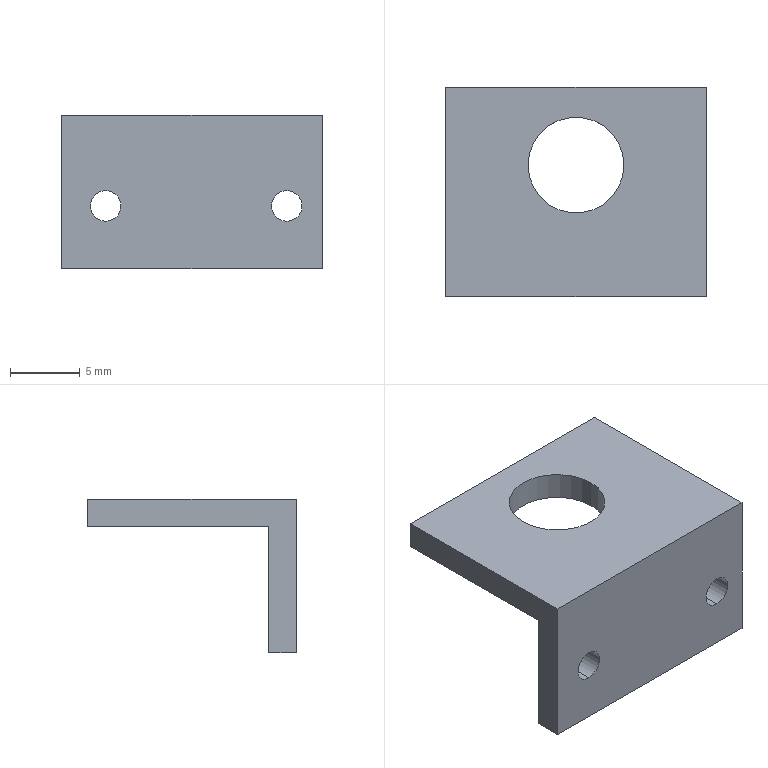Part | SolidWorks | features Extrusion 1, ICE 1 | 1 solid | 14 faces | box 18.701 x 15 x 11.037 mm | volume 809.541 mm3 | plane 8 | cylinder 6 | commonest cylinder face diameters 2.2 x4 6.878 x2
STEP:
#1=CARTESIAN_POINT('',(-3.439,9.421,6.519));
#2=VERTEX_POINT('',#1);
#3=CARTESIAN_POINT('',(3.439,9.421,6.519));
#4=VERTEX_POINT('',#3);
#5=CARTESIAN_POINT('',(0.,9.421,6.519));
#6=DIRECTION('',(0.,0.,1.));
#7=DIRECTION('',(1.,0.,0.));
#8=AXIS2_PLACEMENT_3D('',#5,#6,#7);
#9=CIRCLE('',#8,3.439);
#10=EDGE_CURVE('',#2,#4,#9,.T.);
#11=ORIENTED_EDGE('',*,*,#10,.T.);
#12=CARTESIAN_POINT('',(3.439,9.421,4.519));
#13=VERTEX_POINT('',#12);
#14=CARTESIAN_POINT('',(3.439,9.421,6.519));
#15=DIRECTION('',(0.,0.,-1.));
#16=VECTOR('',#15,1000.);
#17=LINE('',#14,#16);
#18=EDGE_CURVE('',#4,#13,#17,.T.);
#19=ORIENTED_EDGE('',*,*,#18,.T.);
#20=CARTESIAN_POINT('',(-3.439,9.421,4.519));
#21=VERTEX_POINT('',#20);
#22=CARTESIAN_POINT('',(0.,9.421,4.519));
#23=DIRECTION('',(0.,0.,1.));
#24=DIRECTION('',(1.,0.,0.));
#25=AXIS2_PLACEMENT_3D('',#22,#23,#24);
#26=CIRCLE('',#25,3.439);
#27=EDGE_CURVE('',#21,#13,#26,.T.);
#28=ORIENTED_EDGE('',*,*,#27,.F.);
#29=CARTESIAN_POINT('',(-3.439,9.421,6.519));
#30=DIRECTION('',(0.,0.,-1.));
#31=VECTOR('',#30,1000.);
#32=LINE('',#29,#31);
#33=EDGE_CURVE('',#2,#21,#32,.T.);
#34=ORIENTED_EDGE('',*,*,#33,.F.);
#35=EDGE_LOOP('',(#11,#19,#28,#34));
#36=FACE_OUTER_BOUND('',#35,.T.);
#37=CARTESIAN_POINT('',(0.,9.421,6.519));
#38=DIRECTION('',(0.,0.,-1.));
#39=DIRECTION('',(-1.,0.,0.));
#40=AXIS2_PLACEMENT_3D('',#37,#38,#39);
#41=CYLINDRICAL_SURFACE('',#40,3.439);
#42=ADVANCED_FACE('',(#36),#41,.F.);
#43=CARTESIAN_POINT('',(6.803,2.,-1.1));
#44=VERTEX_POINT('',#43);
#45=CARTESIAN_POINT('',(6.803,2.,1.1));
#46=VERTEX_POINT('',#45);
#47=CARTESIAN_POINT('',(6.803,2.,0.));
#48=DIRECTION('',(0.,1.,0.));
#49=DIRECTION('',(0.,0.,1.));
#50=AXIS2_PLACEMENT_3D('',#47,#48,#49);
#51=CIRCLE('',#50,1.1);
#52=EDGE_CURVE('',#44,#46,#51,.T.);
#53=ORIENTED_EDGE('',*,*,#52,.T.);
#54=CARTESIAN_POINT('',(6.803,0.,1.1));
#55=VERTEX_POINT('',#54);
#56=CARTESIAN_POINT('',(6.803,2.,1.1));
#57=DIRECTION('',(0.,-1.,0.));
#58=VECTOR('',#57,1000.);
#59=LINE('',#56,#58);
#60=EDGE_CURVE('',#46,#55,#59,.T.);
#61=ORIENTED_EDGE('',*,*,#60,.T.);
#62=CARTESIAN_POINT('',(6.803,0.,-1.1));
#63=VERTEX_POINT('',#62);
#64=CARTESIAN_POINT('',(6.803,0.,0.));
#65=DIRECTION('',(0.,1.,0.));
#66=DIRECTION('',(0.,0.,1.));
#67=AXIS2_PLACEMENT_3D('',#64,#65,#66);
#68=CIRCLE('',#67,1.1);
#69=EDGE_CURVE('',#63,#55,#68,.T.);
#70=ORIENTED_EDGE('',*,*,#69,.F.);
#71=CARTESIAN_POINT('',(6.803,2.,-1.1));
#72=DIRECTION('',(0.,-1.,0.));
#73=VECTOR('',#72,1000.);
#74=LINE('',#71,#73);
#75=EDGE_CURVE('',#44,#63,#74,.T.);
#76=ORIENTED_EDGE('',*,*,#75,.F.);
#77=EDGE_LOOP('',(#53,#61,#70,#76));
#78=FACE_OUTER_BOUND('',#77,.T.);
#79=CARTESIAN_POINT('',(6.803,2.,0.));
#80=DIRECTION('',(0.,-1.,0.));
#81=DIRECTION('',(0.,0.,-1.));
#82=AXIS2_PLACEMENT_3D('',#79,#80,#81);
#83=CYLINDRICAL_SURFACE('',#82,1.1);
#84=ADVANCED_FACE('',(#78),#83,.F.);
#85=CARTESIAN_POINT('',(-6.197,2.,-1.1));
#86=VERTEX_POINT('',#85);
#87=CARTESIAN_POINT('',(-6.197,2.,1.1));
#88=VERTEX_POINT('',#87);
#89=CARTESIAN_POINT('',(-6.197,2.,0.));
#90=DIRECTION('',(0.,1.,0.));
#91=DIRECTION('',(0.,0.,1.));
#92=AXIS2_PLACEMENT_3D('',#89,#90,#91);
#93=CIRCLE('',#92,1.1);
#94=EDGE_CURVE('',#86,#88,#93,.T.);
#95=ORIENTED_EDGE('',*,*,#94,.T.);
#96=CARTESIAN_POINT('',(-6.197,0.,1.1));
#97=VERTEX_POINT('',#96);
#98=CARTESIAN_POINT('',(-6.197,2.,1.1));
#99=DIRECTION('',(0.,-1.,0.));
#100=VECTOR('',#99,1000.);
#101=LINE('',#98,#100);
#102=EDGE_CURVE('',#88,#97,#101,.T.);
#103=ORIENTED_EDGE('',*,*,#102,.T.);
#104=CARTESIAN_POINT('',(-6.197,0.,-1.1));
#105=VERTEX_POINT('',#104);
#106=CARTESIAN_POINT('',(-6.197,0.,0.));
#107=DIRECTION('',(0.,1.,0.));
#108=DIRECTION('',(0.,0.,1.));
#109=AXIS2_PLACEMENT_3D('',#106,#107,#108);
#110=CIRCLE('',#109,1.1);
#111=EDGE_CURVE('',#105,#97,#110,.T.);
#112=ORIENTED_EDGE('',*,*,#111,.F.);
#113=CARTESIAN_POINT('',(-6.197,2.,-1.1));
#114=DIRECTION('',(0.,-1.,0.));
#115=VECTOR('',#114,1000.);
#116=LINE('',#113,#115);
#117=EDGE_CURVE('',#86,#105,#116,.T.);
#118=ORIENTED_EDGE('',*,*,#117,.F.);
#119=EDGE_LOOP('',(#95,#103,#112,#118));
#120=FACE_OUTER_BOUND('',#119,.T.);
#121=CARTESIAN_POINT('',(-6.197,2.,0.));
#122=DIRECTION('',(0.,-1.,0.));
#123=DIRECTION('',(0.,0.,-1.));
#124=AXIS2_PLACEMENT_3D('',#121,#122,#123);
#125=CYLINDRICAL_SURFACE('',#124,1.1);
#126=ADVANCED_FACE('',(#120),#125,.F.);
#127=CARTESIAN_POINT('',(9.351,2.,4.519));
#128=VERTEX_POINT('',#127);
#129=CARTESIAN_POINT('',(9.351,2.,-4.519));
#130=VERTEX_POINT('',#129);
#131=CARTESIAN_POINT('',(9.351,2.,4.519));
#132=DIRECTION('',(0.,0.,-1.));
#133=VECTOR('',#132,1000.);
#134=LINE('',#131,#133);
#135=EDGE_CURVE('',#128,#130,#134,.T.);
#136=ORIENTED_EDGE('',*,*,#135,.T.);
#137=CARTESIAN_POINT('',(-9.351,2.,-4.519));
#138=VERTEX_POINT('',#137);
#139=CARTESIAN_POINT('',(-9.351,2.,-4.519));
#140=DIRECTION('',(-1.,0.,0.));
#141=VECTOR('',#140,1000.);
#142=LINE('',#139,#141);
#143=EDGE_CURVE('',#130,#138,#142,.T.);
#144=ORIENTED_EDGE('',*,*,#143,.T.);
#145=CARTESIAN_POINT('',(-9.351,2.,4.519));
#146=VERTEX_POINT('',#145);
#147=CARTESIAN_POINT('',(-9.351,2.,4.519));
#148=DIRECTION('',(0.,0.,1.));
#149=VECTOR('',#148,1000.);
#150=LINE('',#147,#149);
#151=EDGE_CURVE('',#138,#146,#150,.T.);
#152=ORIENTED_EDGE('',*,*,#151,.T.);
#153=CARTESIAN_POINT('',(-9.351,2.,4.519));
#154=DIRECTION('',(1.,0.,0.));
#155=VECTOR('',#154,1000.);
#156=LINE('',#153,#155);
#157=EDGE_CURVE('',#146,#128,#156,.T.);
#158=ORIENTED_EDGE('',*,*,#157,.T.);
#159=EDGE_LOOP('',(#136,#144,#152,#158));
#160=FACE_OUTER_BOUND('',#159,.T.);
#161=ORIENTED_EDGE('',*,*,#94,.F.);
#162=CARTESIAN_POINT('',(-6.197,2.,0.));
#163=DIRECTION('',(0.,1.,0.));
#164=DIRECTION('',(0.,0.,1.));
#165=AXIS2_PLACEMENT_3D('',#162,#163,#164);
#166=CIRCLE('',#165,1.1);
#167=EDGE_CURVE('',#88,#86,#166,.T.);
#168=ORIENTED_EDGE('',*,*,#167,.F.);
#169=EDGE_LOOP('',(#161,#168));
#170=FACE_BOUND('',#169,.T.);
#171=ORIENTED_EDGE('',*,*,#52,.F.);
#172=CARTESIAN_POINT('',(6.803,2.,0.));
#173=DIRECTION('',(0.,1.,0.));
#174=DIRECTION('',(0.,0.,1.));
#175=AXIS2_PLACEMENT_3D('',#172,#173,#174);
#176=CIRCLE('',#175,1.1);
#177=EDGE_CURVE('',#46,#44,#176,.T.);
#178=ORIENTED_EDGE('',*,*,#177,.F.);
#179=EDGE_LOOP('',(#171,#178));
#180=FACE_BOUND('',#179,.T.);
#181=CARTESIAN_POINT('',(0.,2.,0.));
#182=DIRECTION('',(0.,-1.,0.));
#183=DIRECTION('',(0.,0.,-1.));
#184=AXIS2_PLACEMENT_3D('',#181,#182,#183);
#185=PLANE('',#184);
#186=ADVANCED_FACE('',(#160,#170,#180),#185,.F.);
#187=ORIENTED_EDGE('',*,*,#111,.T.);
#188=CARTESIAN_POINT('',(-6.197,0.,0.));
#189=DIRECTION('',(0.,1.,0.));
#190=DIRECTION('',(0.,0.,1.));
#191=AXIS2_PLACEMENT_3D('',#188,#189,#190);
#192=CIRCLE('',#191,1.1);
#193=EDGE_CURVE('',#97,#105,#192,.T.);
#194=ORIENTED_EDGE('',*,*,#193,.T.);
#195=EDGE_LOOP('',(#187,#194));
#196=FACE_BOUND('',#195,.T.);
#197=CARTESIAN_POINT('',(9.351,0.,6.519));
#198=VERTEX_POINT('',#197);
#199=CARTESIAN_POINT('',(9.351,0.,-4.519));
#200=VERTEX_POINT('',#199);
#201=CARTESIAN_POINT('',(9.351,0.,4.519));
#202=DIRECTION('',(0.,0.,-1.));
#203=VECTOR('',#202,1000.);
#204=LINE('',#201,#203);
#205=EDGE_CURVE('',#198,#200,#204,.T.);
#206=ORIENTED_EDGE('',*,*,#205,.F.);
#207=CARTESIAN_POINT('',(-9.351,0.,6.519));
#208=VERTEX_POINT('',#207);
#209=CARTESIAN_POINT('',(-9.351,0.,6.519));
#210=DIRECTION('',(1.,0.,0.));
#211=VECTOR('',#210,1000.);
#212=LINE('',#209,#211);
#213=EDGE_CURVE('',#208,#198,#212,.T.);
#214=ORIENTED_EDGE('',*,*,#213,.F.);
#215=CARTESIAN_POINT('',(-9.351,0.,-4.519));
#216=VERTEX_POINT('',#215);
#217=CARTESIAN_POINT('',(-9.351,0.,4.519));
#218=DIRECTION('',(0.,0.,1.));
#219=VECTOR('',#218,1000.);
#220=LINE('',#217,#219);
#221=EDGE_CURVE('',#216,#208,#220,.T.);
#222=ORIENTED_EDGE('',*,*,#221,.F.);
#223=CARTESIAN_POINT('',(-9.351,0.,-4.519));
#224=DIRECTION('',(-1.,0.,0.));
#225=VECTOR('',#224,1000.);
#226=LINE('',#223,#225);
#227=EDGE_CURVE('',#200,#216,#226,.T.);
#228=ORIENTED_EDGE('',*,*,#227,.F.);
#229=EDGE_LOOP('',(#206,#214,#222,#228));
#230=FACE_OUTER_BOUND('',#229,.T.);
#231=ORIENTED_EDGE('',*,*,#69,.T.);
#232=CARTESIAN_POINT('',(6.803,0.,0.));
#233=DIRECTION('',(0.,1.,0.));
#234=DIRECTION('',(0.,0.,1.));
#235=AXIS2_PLACEMENT_3D('',#232,#233,#234);
#236=CIRCLE('',#235,1.1);
#237=EDGE_CURVE('',#55,#63,#236,.T.);
#238=ORIENTED_EDGE('',*,*,#237,.T.);
#239=EDGE_LOOP('',(#231,#238));
#240=FACE_BOUND('',#239,.T.);
#241=CARTESIAN_POINT('',(0.,0.,0.));
#242=DIRECTION('',(0.,-1.,0.));
#243=DIRECTION('',(0.,0.,-1.));
#244=AXIS2_PLACEMENT_3D('',#241,#242,#243);
#245=PLANE('',#244);
#246=ADVANCED_FACE('',(#196,#230,#240),#245,.T.);
#247=ORIENTED_EDGE('',*,*,#205,.T.);
#248=CARTESIAN_POINT('',(9.351,2.,-4.519));
#249=DIRECTION('',(0.,-1.,0.));
#250=VECTOR('',#249,1000.);
#251=LINE('',#248,#250);
#252=EDGE_CURVE('',#130,#200,#251,.T.);
#253=ORIENTED_EDGE('',*,*,#252,.F.);
#254=ORIENTED_EDGE('',*,*,#135,.F.);
#255=CARTESIAN_POINT('',(9.351,15.,4.519));
#256=VERTEX_POINT('',#255);
#257=CARTESIAN_POINT('',(9.351,0.,4.519));
#258=DIRECTION('',(0.,1.,0.));
#259=VECTOR('',#258,1000.);
#260=LINE('',#257,#259);
#261=EDGE_CURVE('',#128,#256,#260,.T.);
#262=ORIENTED_EDGE('',*,*,#261,.T.);
#263=CARTESIAN_POINT('',(9.351,15.,6.519));
#264=VERTEX_POINT('',#263);
#265=CARTESIAN_POINT('',(9.351,15.,6.519));
#266=DIRECTION('',(0.,0.,-1.));
#267=VECTOR('',#266,1000.);
#268=LINE('',#265,#267);
#269=EDGE_CURVE('',#264,#256,#268,.T.);
#270=ORIENTED_EDGE('',*,*,#269,.F.);
#271=CARTESIAN_POINT('',(9.351,0.,6.519));
#272=DIRECTION('',(0.,1.,0.));
#273=VECTOR('',#272,1000.);
#274=LINE('',#271,#273);
#275=EDGE_CURVE('',#198,#264,#274,.T.);
#276=ORIENTED_EDGE('',*,*,#275,.F.);
#277=EDGE_LOOP('',(#247,#253,#254,#262,#270,#276));
#278=FACE_OUTER_BOUND('',#277,.T.);
#279=CARTESIAN_POINT('',(9.351,2.,4.519));
#280=DIRECTION('',(-1.,0.,0.));
#281=DIRECTION('',(0.,0.,1.));
#282=AXIS2_PLACEMENT_3D('',#279,#280,#281);
#283=PLANE('',#282);
#284=ADVANCED_FACE('',(#278),#283,.F.);
#285=ORIENTED_EDGE('',*,*,#227,.T.);
#286=CARTESIAN_POINT('',(-9.351,2.,-4.519));
#287=DIRECTION('',(0.,-1.,0.));
#288=VECTOR('',#287,1000.);
#289=LINE('',#286,#288);
#290=EDGE_CURVE('',#138,#216,#289,.T.);
#291=ORIENTED_EDGE('',*,*,#290,.F.);
#292=ORIENTED_EDGE('',*,*,#143,.F.);
#293=ORIENTED_EDGE('',*,*,#252,.T.);
#294=EDGE_LOOP('',(#285,#291,#292,#293));
#295=FACE_OUTER_BOUND('',#294,.T.);
#296=CARTESIAN_POINT('',(-9.351,2.,-4.519));
#297=DIRECTION('',(0.,0.,1.));
#298=DIRECTION('',(1.,0.,0.));
#299=AXIS2_PLACEMENT_3D('',#296,#297,#298);
#300=PLANE('',#299);
#301=ADVANCED_FACE('',(#295),#300,.F.);
#302=ORIENTED_EDGE('',*,*,#221,.T.);
#303=CARTESIAN_POINT('',(-9.351,15.,6.519));
#304=VERTEX_POINT('',#303);
#305=CARTESIAN_POINT('',(-9.351,0.,6.519));
#306=DIRECTION('',(0.,-1.,0.));
#307=VECTOR('',#306,1000.);
#308=LINE('',#305,#307);
#309=EDGE_CURVE('',#304,#208,#308,.T.);
#310=ORIENTED_EDGE('',*,*,#309,.F.);
#311=CARTESIAN_POINT('',(-9.351,15.,4.519));
#312=VERTEX_POINT('',#311);
#313=CARTESIAN_POINT('',(-9.351,15.,6.519));
#314=DIRECTION('',(0.,0.,-1.));
#315=VECTOR('',#314,1000.);
#316=LINE('',#313,#315);
#317=EDGE_CURVE('',#304,#312,#316,.T.);
#318=ORIENTED_EDGE('',*,*,#317,.T.);
#319=CARTESIAN_POINT('',(-9.351,0.,4.519));
#320=DIRECTION('',(0.,-1.,0.));
#321=VECTOR('',#320,1000.);
#322=LINE('',#319,#321);
#323=EDGE_CURVE('',#312,#146,#322,.T.);
#324=ORIENTED_EDGE('',*,*,#323,.T.);
#325=ORIENTED_EDGE('',*,*,#151,.F.);
#326=ORIENTED_EDGE('',*,*,#290,.T.);
#327=EDGE_LOOP('',(#302,#310,#318,#324,#325,#326));
#328=FACE_OUTER_BOUND('',#327,.T.);
#329=CARTESIAN_POINT('',(-9.351,2.,4.519));
#330=DIRECTION('',(1.,0.,0.));
#331=DIRECTION('',(0.,0.,-1.));
#332=AXIS2_PLACEMENT_3D('',#329,#330,#331);
#333=PLANE('',#332);
#334=ADVANCED_FACE('',(#328),#333,.F.);
#335=ORIENTED_EDGE('',*,*,#102,.F.);
#336=ORIENTED_EDGE('',*,*,#167,.T.);
#337=ORIENTED_EDGE('',*,*,#117,.T.);
#338=ORIENTED_EDGE('',*,*,#193,.F.);
#339=EDGE_LOOP('',(#335,#336,#337,#338));
#340=FACE_OUTER_BOUND('',#339,.T.);
#341=CARTESIAN_POINT('',(-6.197,2.,0.));
#342=DIRECTION('',(0.,-1.,0.));
#343=DIRECTION('',(0.,0.,-1.));
#344=AXIS2_PLACEMENT_3D('',#341,#342,#343);
#345=CYLINDRICAL_SURFACE('',#344,1.1);
#346=ADVANCED_FACE('',(#340),#345,.F.);
#347=ORIENTED_EDGE('',*,*,#60,.F.);
#348=ORIENTED_EDGE('',*,*,#177,.T.);
#349=ORIENTED_EDGE('',*,*,#75,.T.);
#350=ORIENTED_EDGE('',*,*,#237,.F.);
#351=EDGE_LOOP('',(#347,#348,#349,#350));
#352=FACE_OUTER_BOUND('',#351,.T.);
#353=CARTESIAN_POINT('',(6.803,2.,0.));
#354=DIRECTION('',(0.,-1.,0.));
#355=DIRECTION('',(0.,0.,-1.));
#356=AXIS2_PLACEMENT_3D('',#353,#354,#355);
#357=CYLINDRICAL_SURFACE('',#356,1.1);
#358=ADVANCED_FACE('',(#352),#357,.F.);
#359=ORIENTED_EDGE('',*,*,#27,.T.);
#360=CARTESIAN_POINT('',(0.,9.421,4.519));
#361=DIRECTION('',(0.,0.,1.));
#362=DIRECTION('',(1.,0.,0.));
#363=AXIS2_PLACEMENT_3D('',#360,#361,#362);
#364=CIRCLE('',#363,3.439);
#365=EDGE_CURVE('',#13,#21,#364,.T.);
#366=ORIENTED_EDGE('',*,*,#365,.T.);
#367=EDGE_LOOP('',(#359,#366));
#368=FACE_BOUND('',#367,.T.);
#369=ORIENTED_EDGE('',*,*,#157,.F.);
#370=ORIENTED_EDGE('',*,*,#323,.F.);
#371=CARTESIAN_POINT('',(-9.351,15.,4.519));
#372=DIRECTION('',(-1.,0.,0.));
#373=VECTOR('',#372,1000.);
#374=LINE('',#371,#373);
#375=EDGE_CURVE('',#256,#312,#374,.T.);
#376=ORIENTED_EDGE('',*,*,#375,.F.);
#377=ORIENTED_EDGE('',*,*,#261,.F.);
#378=EDGE_LOOP('',(#369,#370,#376,#377));
#379=FACE_OUTER_BOUND('',#378,.T.);
#380=CARTESIAN_POINT('',(0.,0.,4.519));
#381=DIRECTION('',(0.,0.,-1.));
#382=DIRECTION('',(-1.,0.,0.));
#383=AXIS2_PLACEMENT_3D('',#380,#381,#382);
#384=PLANE('',#383);
#385=ADVANCED_FACE('',(#368,#379),#384,.T.);
#386=ORIENTED_EDGE('',*,*,#309,.T.);
#387=ORIENTED_EDGE('',*,*,#213,.T.);
#388=ORIENTED_EDGE('',*,*,#275,.T.);
#389=CARTESIAN_POINT('',(-9.351,15.,6.519));
#390=DIRECTION('',(-1.,0.,0.));
#391=VECTOR('',#390,1000.);
#392=LINE('',#389,#391);
#393=EDGE_CURVE('',#264,#304,#392,.T.);
#394=ORIENTED_EDGE('',*,*,#393,.T.);
#395=EDGE_LOOP('',(#386,#387,#388,#394));
#396=FACE_OUTER_BOUND('',#395,.T.);
#397=ORIENTED_EDGE('',*,*,#10,.F.);
#398=CARTESIAN_POINT('',(0.,9.421,6.519));
#399=DIRECTION('',(0.,0.,1.));
#400=DIRECTION('',(1.,0.,0.));
#401=AXIS2_PLACEMENT_3D('',#398,#399,#400);
#402=CIRCLE('',#401,3.439);
#403=EDGE_CURVE('',#4,#2,#402,.T.);
#404=ORIENTED_EDGE('',*,*,#403,.F.);
#405=EDGE_LOOP('',(#397,#404));
#406=FACE_BOUND('',#405,.T.);
#407=CARTESIAN_POINT('',(0.,0.,6.519));
#408=DIRECTION('',(0.,0.,-1.));
#409=DIRECTION('',(-1.,0.,0.));
#410=AXIS2_PLACEMENT_3D('',#407,#408,#409);
#411=PLANE('',#410);
#412=ADVANCED_FACE('',(#396,#406),#411,.F.);
#413=ORIENTED_EDGE('',*,*,#375,.T.);
#414=ORIENTED_EDGE('',*,*,#317,.F.);
#415=ORIENTED_EDGE('',*,*,#393,.F.);
#416=ORIENTED_EDGE('',*,*,#269,.T.);
#417=EDGE_LOOP('',(#413,#414,#415,#416));
#418=FACE_OUTER_BOUND('',#417,.T.);
#419=CARTESIAN_POINT('',(-9.351,15.,6.519));
#420=DIRECTION('',(0.,-1.,0.));
#421=DIRECTION('',(0.,0.,-1.));
#422=AXIS2_PLACEMENT_3D('',#419,#420,#421);
#423=PLANE('',#422);
#424=ADVANCED_FACE('',(#418),#423,.F.);
#425=ORIENTED_EDGE('',*,*,#18,.F.);
#426=ORIENTED_EDGE('',*,*,#403,.T.);
#427=ORIENTED_EDGE('',*,*,#33,.T.);
#428=ORIENTED_EDGE('',*,*,#365,.F.);
#429=EDGE_LOOP('',(#425,#426,#427,#428));
#430=FACE_OUTER_BOUND('',#429,.T.);
#431=CARTESIAN_POINT('',(0.,9.421,6.519));
#432=DIRECTION('',(0.,0.,-1.));
#433=DIRECTION('',(-1.,0.,0.));
#434=AXIS2_PLACEMENT_3D('',#431,#432,#433);
#435=CYLINDRICAL_SURFACE('',#434,3.439);
#436=ADVANCED_FACE('',(#430),#435,.F.);
#437=CLOSED_SHELL('',(#42,#84,#126,#186,#246,#284,#301,#334,#346,#358,#385,#412,#424,#436));
#438=MANIFOLD_SOLID_BREP('',#437);
#439=CARTESIAN_POINT('',(0.,0.,0.));
#440=DIRECTION('',(0.,0.,1.));
#441=DIRECTION('',(1.,0.,0.));
#442=AXIS2_PLACEMENT_3D('',#439,#440,#441);
#443=(LENGTH_UNIT()NAMED_UNIT(*)SI_UNIT(.MILLI.,.METRE.));
#444=UNCERTAINTY_MEASURE_WITH_UNIT(LENGTH_MEASURE(0.00001),#443,'','');
#445=(NAMED_UNIT(*)PLANE_ANGLE_UNIT()SI_UNIT($,.RADIAN.));
#446=(NAMED_UNIT(*)SI_UNIT($,.STERADIAN.)SOLID_ANGLE_UNIT());
#447=(GEOMETRIC_REPRESENTATION_CONTEXT(3)GLOBAL_UNCERTAINTY_ASSIGNED_CONTEXT((#444))GLOBAL_UNIT_ASSIGNED_CONTEXT((#443,#445,#446))REPRESENTATION_CONTEXT('',''));
#448=ADVANCED_BREP_SHAPE_REPRESENTATION('',(#438,#442),#447);